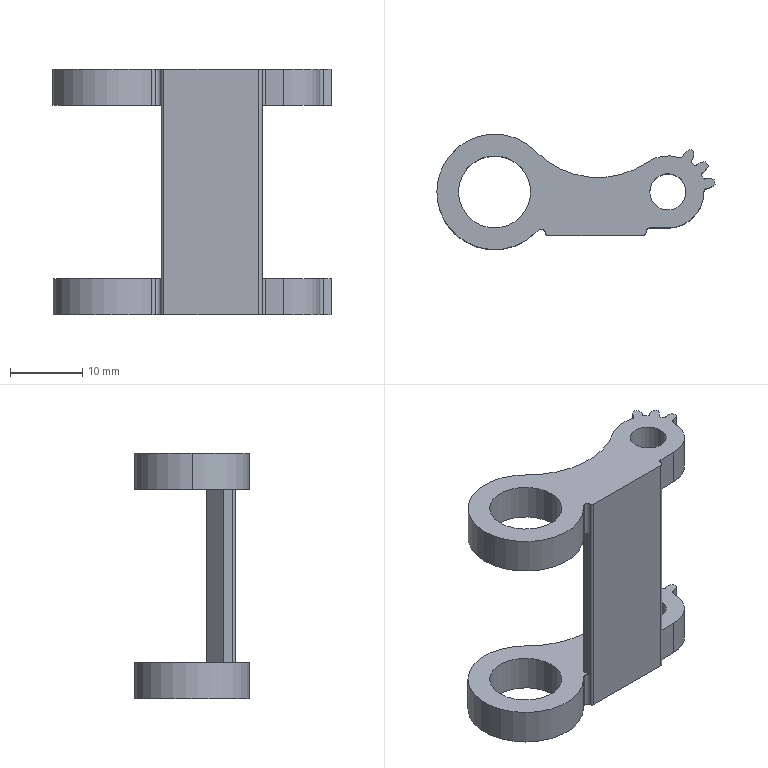Part | SolidWorks | features HoleWzd 4, ICE 4, Fillet 2, RefSurface 2, ThickenCut 2, Extrusion 1 | 1 solid | 58 faces | box 38.562 x 16 x 34 mm | volume 4236 mm3 | cylinder 35 | plane 15 | spline 8 | commonest cylinder face diameters 1 x9 10 x8 13.28 x6 5 x4 16 x3 4 x2